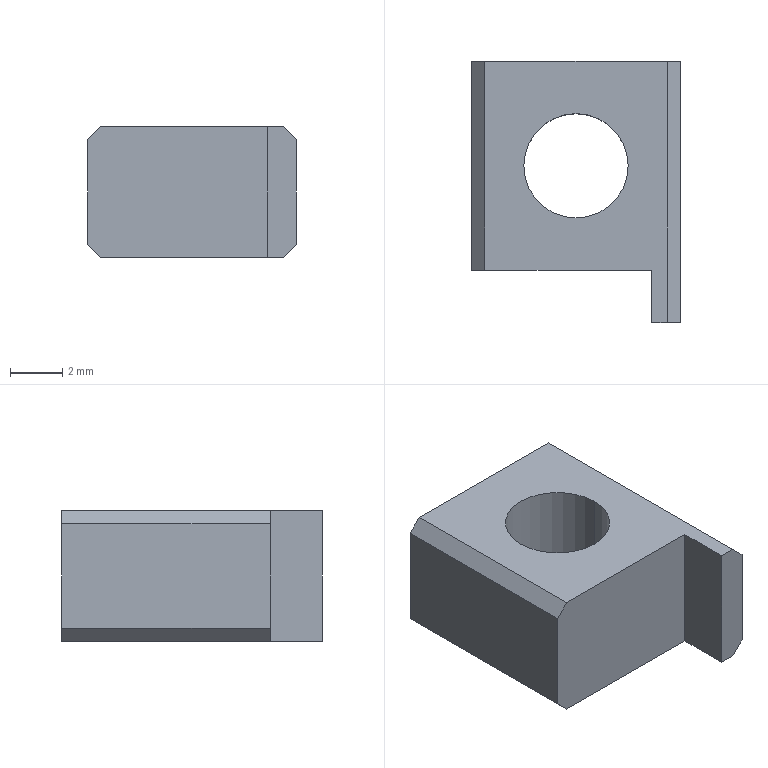Part | NX | 1 solid | 14 faces | box 8 x 10 x 5 mm | volume 263.668 mm3 | plane 12 | cylinder 2 | commonest cylinder face diameters 4 x2
STEP:
#1=CARTESIAN_POINT('',(0.5,10.,0.));
#2=VERTEX_POINT('',#1);
#3=CARTESIAN_POINT('',(7.5,10.,0.));
#4=VERTEX_POINT('',#3);
#5=CARTESIAN_POINT('',(0.,10.,0.));
#6=DIRECTION('',(1.,0.,0.));
#7=VECTOR('',#6,1000.);
#8=LINE('',#5,#7);
#9=EDGE_CURVE('',#2,#4,#8,.T.);
#10=ORIENTED_EDGE('',*,*,#9,.T.);
#11=CARTESIAN_POINT('',(7.5,0.,0.));
#12=VERTEX_POINT('',#11);
#13=CARTESIAN_POINT('',(7.5,0.,0.));
#14=DIRECTION('',(0.,-1.,0.));
#15=VECTOR('',#14,1000.);
#16=LINE('',#13,#15);
#17=EDGE_CURVE('',#4,#12,#16,.T.);
#18=ORIENTED_EDGE('',*,*,#17,.T.);
#19=CARTESIAN_POINT('',(6.9,0.,0.));
#20=VERTEX_POINT('',#19);
#21=CARTESIAN_POINT('',(0.,0.,0.));
#22=DIRECTION('',(1.,0.,0.));
#23=VECTOR('',#22,1000.);
#24=LINE('',#21,#23);
#25=EDGE_CURVE('',#20,#12,#24,.T.);
#26=ORIENTED_EDGE('',*,*,#25,.F.);
#27=CARTESIAN_POINT('',(6.9,2.,0.));
#28=VERTEX_POINT('',#27);
#29=CARTESIAN_POINT('',(6.9,0.,0.));
#30=DIRECTION('',(0.,1.,0.));
#31=VECTOR('',#30,1000.);
#32=LINE('',#29,#31);
#33=EDGE_CURVE('',#20,#28,#32,.T.);
#34=ORIENTED_EDGE('',*,*,#33,.T.);
#35=CARTESIAN_POINT('',(0.5,2.,0.));
#36=VERTEX_POINT('',#35);
#37=CARTESIAN_POINT('',(0.,2.,0.));
#38=DIRECTION('',(-1.,0.,0.));
#39=VECTOR('',#38,1000.);
#40=LINE('',#37,#39);
#41=EDGE_CURVE('',#28,#36,#40,.T.);
#42=ORIENTED_EDGE('',*,*,#41,.T.);
#43=CARTESIAN_POINT('',(0.5,0.,0.));
#44=DIRECTION('',(0.,1.,0.));
#45=VECTOR('',#44,1000.);
#46=LINE('',#43,#45);
#47=EDGE_CURVE('',#36,#2,#46,.T.);
#48=ORIENTED_EDGE('',*,*,#47,.T.);
#49=EDGE_LOOP('',(#10,#18,#26,#34,#42,#48));
#50=FACE_BOUND('',#49,.T.);
#51=CARTESIAN_POINT('',(6.,6.,0.));
#52=VERTEX_POINT('',#51);
#53=CARTESIAN_POINT('',(2.,6.,0.));
#54=VERTEX_POINT('',#53);
#55=CARTESIAN_POINT('',(4.,6.,0.));
#56=DIRECTION('',(0.,0.,-1.));
#57=DIRECTION('',(-1.,0.,0.));
#58=AXIS2_PLACEMENT_3D('',#55,#56,#57);
#59=CIRCLE('',#58,2.);
#60=EDGE_CURVE('',#52,#54,#59,.T.);
#61=ORIENTED_EDGE('',*,*,#60,.F.);
#62=CARTESIAN_POINT('',(4.,6.,0.));
#63=DIRECTION('',(0.,0.,-1.));
#64=DIRECTION('',(-1.,0.,0.));
#65=AXIS2_PLACEMENT_3D('',#62,#63,#64);
#66=CIRCLE('',#65,2.);
#67=EDGE_CURVE('',#54,#52,#66,.T.);
#68=ORIENTED_EDGE('',*,*,#67,.F.);
#69=EDGE_LOOP('',(#61,#68));
#70=FACE_BOUND('',#69,.T.);
#71=CARTESIAN_POINT('',(0.,0.,0.));
#72=DIRECTION('',(0.,0.,1.));
#73=DIRECTION('',(1.,0.,0.));
#74=AXIS2_PLACEMENT_3D('',#71,#72,#73);
#75=PLANE('',#74);
#76=ADVANCED_FACE('',(#50,#70),#75,.F.);
#77=ORIENTED_EDGE('',*,*,#33,.F.);
#78=CARTESIAN_POINT('',(6.9,0.,5.));
#79=VERTEX_POINT('',#78);
#80=CARTESIAN_POINT('',(6.9,0.,0.));
#81=DIRECTION('',(0.,0.,1.));
#82=VECTOR('',#81,1000.);
#83=LINE('',#80,#82);
#84=EDGE_CURVE('',#20,#79,#83,.T.);
#85=ORIENTED_EDGE('',*,*,#84,.T.);
#86=CARTESIAN_POINT('',(6.9,2.,5.));
#87=VERTEX_POINT('',#86);
#88=CARTESIAN_POINT('',(6.9,0.,5.));
#89=DIRECTION('',(0.,1.,0.));
#90=VECTOR('',#89,1000.);
#91=LINE('',#88,#90);
#92=EDGE_CURVE('',#79,#87,#91,.T.);
#93=ORIENTED_EDGE('',*,*,#92,.T.);
#94=CARTESIAN_POINT('',(6.9,2.,0.));
#95=DIRECTION('',(0.,0.,1.));
#96=VECTOR('',#95,1000.);
#97=LINE('',#94,#96);
#98=EDGE_CURVE('',#28,#87,#97,.T.);
#99=ORIENTED_EDGE('',*,*,#98,.F.);
#100=EDGE_LOOP('',(#77,#85,#93,#99));
#101=FACE_BOUND('',#100,.T.);
#102=CARTESIAN_POINT('',(6.9,0.,5.));
#103=DIRECTION('',(1.,0.,0.));
#104=DIRECTION('',(0.,1.,0.));
#105=AXIS2_PLACEMENT_3D('',#102,#103,#104);
#106=PLANE('',#105);
#107=ADVANCED_FACE('',(#101),#106,.F.);
#108=ORIENTED_EDGE('',*,*,#41,.F.);
#109=ORIENTED_EDGE('',*,*,#98,.T.);
#110=CARTESIAN_POINT('',(0.5,2.,5.));
#111=VERTEX_POINT('',#110);
#112=CARTESIAN_POINT('',(0.,2.,5.));
#113=DIRECTION('',(-1.,0.,0.));
#114=VECTOR('',#113,1000.);
#115=LINE('',#112,#114);
#116=EDGE_CURVE('',#87,#111,#115,.T.);
#117=ORIENTED_EDGE('',*,*,#116,.T.);
#118=CARTESIAN_POINT('',(0.,2.,4.5));
#119=VERTEX_POINT('',#118);
#120=CARTESIAN_POINT('',(-4.5,2.,0.));
#121=DIRECTION('',(-0.7071,0.,-0.7071));
#122=VECTOR('',#121,1000.);
#123=LINE('',#120,#122);
#124=EDGE_CURVE('',#111,#119,#123,.T.);
#125=ORIENTED_EDGE('',*,*,#124,.T.);
#126=CARTESIAN_POINT('',(0.,2.,0.5));
#127=VERTEX_POINT('',#126);
#128=CARTESIAN_POINT('',(0.,2.,0.));
#129=DIRECTION('',(0.,0.,-1.));
#130=VECTOR('',#129,1000.);
#131=LINE('',#128,#130);
#132=EDGE_CURVE('',#119,#127,#131,.T.);
#133=ORIENTED_EDGE('',*,*,#132,.T.);
#134=CARTESIAN_POINT('',(0.5,2.,0.));
#135=DIRECTION('',(0.7071,0.,-0.7071));
#136=VECTOR('',#135,1000.);
#137=LINE('',#134,#136);
#138=EDGE_CURVE('',#127,#36,#137,.T.);
#139=ORIENTED_EDGE('',*,*,#138,.T.);
#140=EDGE_LOOP('',(#108,#109,#117,#125,#133,#139));
#141=FACE_BOUND('',#140,.T.);
#142=CARTESIAN_POINT('',(7.,2.,5.));
#143=DIRECTION('',(0.,1.,0.));
#144=DIRECTION('',(1.,0.,0.));
#145=AXIS2_PLACEMENT_3D('',#142,#143,#144);
#146=PLANE('',#145);
#147=ADVANCED_FACE('',(#141),#146,.F.);
#148=CARTESIAN_POINT('',(0.,10.,4.5));
#149=VERTEX_POINT('',#148);
#150=CARTESIAN_POINT('',(0.,0.,4.5));
#151=DIRECTION('',(0.,-1.,0.));
#152=VECTOR('',#151,1000.);
#153=LINE('',#150,#152);
#154=EDGE_CURVE('',#149,#119,#153,.T.);
#155=ORIENTED_EDGE('',*,*,#154,.F.);
#156=CARTESIAN_POINT('',(0.,10.,0.5));
#157=VERTEX_POINT('',#156);
#158=CARTESIAN_POINT('',(0.,10.,0.));
#159=DIRECTION('',(0.,0.,-1.));
#160=VECTOR('',#159,1000.);
#161=LINE('',#158,#160);
#162=EDGE_CURVE('',#149,#157,#161,.T.);
#163=ORIENTED_EDGE('',*,*,#162,.T.);
#164=CARTESIAN_POINT('',(0.,0.,0.5));
#165=DIRECTION('',(0.,-1.,0.));
#166=VECTOR('',#165,1000.);
#167=LINE('',#164,#166);
#168=EDGE_CURVE('',#157,#127,#167,.T.);
#169=ORIENTED_EDGE('',*,*,#168,.T.);
#170=ORIENTED_EDGE('',*,*,#132,.F.);
#171=EDGE_LOOP('',(#155,#163,#169,#170));
#172=FACE_BOUND('',#171,.T.);
#173=CARTESIAN_POINT('',(0.,10.,0.));
#174=DIRECTION('',(-1.,0.,0.));
#175=DIRECTION('',(0.,0.,1.));
#176=AXIS2_PLACEMENT_3D('',#173,#174,#175);
#177=PLANE('',#176);
#178=ADVANCED_FACE('',(#172),#177,.T.);
#179=CARTESIAN_POINT('',(8.,10.,0.5));
#180=VERTEX_POINT('',#179);
#181=CARTESIAN_POINT('',(7.5,10.,0.));
#182=DIRECTION('',(-0.7071,0.,-0.7071));
#183=VECTOR('',#182,1000.);
#184=LINE('',#181,#183);
#185=EDGE_CURVE('',#180,#4,#184,.T.);
#186=ORIENTED_EDGE('',*,*,#185,.T.);
#187=ORIENTED_EDGE('',*,*,#9,.F.);
#188=CARTESIAN_POINT('',(0.5,10.,0.));
#189=DIRECTION('',(-0.7071,0.,0.7071));
#190=VECTOR('',#189,1000.);
#191=LINE('',#188,#190);
#192=EDGE_CURVE('',#2,#157,#191,.T.);
#193=ORIENTED_EDGE('',*,*,#192,.T.);
#194=ORIENTED_EDGE('',*,*,#162,.F.);
#195=CARTESIAN_POINT('',(0.5,10.,5.));
#196=VERTEX_POINT('',#195);
#197=CARTESIAN_POINT('',(-4.5,10.,0.));
#198=DIRECTION('',(-0.7071,0.,-0.7071));
#199=VECTOR('',#198,1000.);
#200=LINE('',#197,#199);
#201=EDGE_CURVE('',#196,#149,#200,.T.);
#202=ORIENTED_EDGE('',*,*,#201,.F.);
#203=CARTESIAN_POINT('',(7.5,10.,5.));
#204=VERTEX_POINT('',#203);
#205=CARTESIAN_POINT('',(0.,10.,5.));
#206=DIRECTION('',(1.,0.,0.));
#207=VECTOR('',#206,1000.);
#208=LINE('',#205,#207);
#209=EDGE_CURVE('',#196,#204,#208,.T.);
#210=ORIENTED_EDGE('',*,*,#209,.T.);
#211=CARTESIAN_POINT('',(8.,10.,4.5));
#212=VERTEX_POINT('',#211);
#213=CARTESIAN_POINT('',(12.5,10.,0.));
#214=DIRECTION('',(-0.7071,0.,0.7071));
#215=VECTOR('',#214,1000.);
#216=LINE('',#213,#215);
#217=EDGE_CURVE('',#212,#204,#216,.T.);
#218=ORIENTED_EDGE('',*,*,#217,.F.);
#219=CARTESIAN_POINT('',(8.,10.,0.));
#220=DIRECTION('',(0.,0.,1.));
#221=VECTOR('',#220,1000.);
#222=LINE('',#219,#221);
#223=EDGE_CURVE('',#180,#212,#222,.T.);
#224=ORIENTED_EDGE('',*,*,#223,.F.);
#225=EDGE_LOOP('',(#186,#187,#193,#194,#202,#210,#218,#224));
#226=FACE_BOUND('',#225,.T.);
#227=CARTESIAN_POINT('',(8.,10.,0.));
#228=DIRECTION('',(0.,1.,0.));
#229=DIRECTION('',(1.,0.,0.));
#230=AXIS2_PLACEMENT_3D('',#227,#228,#229);
#231=PLANE('',#230);
#232=ADVANCED_FACE('',(#226),#231,.T.);
#233=CARTESIAN_POINT('',(8.,0.,4.5));
#234=VERTEX_POINT('',#233);
#235=CARTESIAN_POINT('',(8.,0.,4.5));
#236=DIRECTION('',(0.,1.,0.));
#237=VECTOR('',#236,1000.);
#238=LINE('',#235,#237);
#239=EDGE_CURVE('',#234,#212,#238,.T.);
#240=ORIENTED_EDGE('',*,*,#239,.F.);
#241=CARTESIAN_POINT('',(8.,0.,0.5));
#242=VERTEX_POINT('',#241);
#243=CARTESIAN_POINT('',(8.,0.,0.));
#244=DIRECTION('',(0.,0.,-1.));
#245=VECTOR('',#244,1000.);
#246=LINE('',#243,#245);
#247=EDGE_CURVE('',#234,#242,#246,.T.);
#248=ORIENTED_EDGE('',*,*,#247,.T.);
#249=CARTESIAN_POINT('',(8.,0.,0.5));
#250=DIRECTION('',(0.,1.,0.));
#251=VECTOR('',#250,1000.);
#252=LINE('',#249,#251);
#253=EDGE_CURVE('',#242,#180,#252,.T.);
#254=ORIENTED_EDGE('',*,*,#253,.T.);
#255=ORIENTED_EDGE('',*,*,#223,.T.);
#256=EDGE_LOOP('',(#240,#248,#254,#255));
#257=FACE_BOUND('',#256,.T.);
#258=CARTESIAN_POINT('',(8.,0.,0.));
#259=DIRECTION('',(1.,0.,0.));
#260=DIRECTION('',(0.,1.,0.));
#261=AXIS2_PLACEMENT_3D('',#258,#259,#260);
#262=PLANE('',#261);
#263=ADVANCED_FACE('',(#257),#262,.T.);
#264=ORIENTED_EDGE('',*,*,#84,.F.);
#265=ORIENTED_EDGE('',*,*,#25,.T.);
#266=CARTESIAN_POINT('',(7.5,0.,0.));
#267=DIRECTION('',(-0.7071,0.,-0.7071));
#268=VECTOR('',#267,1000.);
#269=LINE('',#266,#268);
#270=EDGE_CURVE('',#242,#12,#269,.T.);
#271=ORIENTED_EDGE('',*,*,#270,.F.);
#272=ORIENTED_EDGE('',*,*,#247,.F.);
#273=CARTESIAN_POINT('',(7.5,0.,5.));
#274=VERTEX_POINT('',#273);
#275=CARTESIAN_POINT('',(12.5,0.,0.));
#276=DIRECTION('',(0.7071,0.,-0.7071));
#277=VECTOR('',#276,1000.);
#278=LINE('',#275,#277);
#279=EDGE_CURVE('',#274,#234,#278,.T.);
#280=ORIENTED_EDGE('',*,*,#279,.F.);
#281=CARTESIAN_POINT('',(0.,0.,5.));
#282=DIRECTION('',(1.,0.,0.));
#283=VECTOR('',#282,1000.);
#284=LINE('',#281,#283);
#285=EDGE_CURVE('',#79,#274,#284,.T.);
#286=ORIENTED_EDGE('',*,*,#285,.F.);
#287=EDGE_LOOP('',(#264,#265,#271,#272,#280,#286));
#288=FACE_BOUND('',#287,.T.);
#289=CARTESIAN_POINT('',(0.,0.,0.));
#290=DIRECTION('',(0.,-1.,0.));
#291=DIRECTION('',(0.,0.,-1.));
#292=AXIS2_PLACEMENT_3D('',#289,#290,#291);
#293=PLANE('',#292);
#294=ADVANCED_FACE('',(#288),#293,.T.);
#295=ORIENTED_EDGE('',*,*,#209,.F.);
#296=CARTESIAN_POINT('',(0.5,0.,5.));
#297=DIRECTION('',(0.,1.,0.));
#298=VECTOR('',#297,1000.);
#299=LINE('',#296,#298);
#300=EDGE_CURVE('',#111,#196,#299,.T.);
#301=ORIENTED_EDGE('',*,*,#300,.F.);
#302=ORIENTED_EDGE('',*,*,#116,.F.);
#303=ORIENTED_EDGE('',*,*,#92,.F.);
#304=ORIENTED_EDGE('',*,*,#285,.T.);
#305=CARTESIAN_POINT('',(7.5,0.,5.));
#306=DIRECTION('',(0.,-1.,0.));
#307=VECTOR('',#306,1000.);
#308=LINE('',#305,#307);
#309=EDGE_CURVE('',#204,#274,#308,.T.);
#310=ORIENTED_EDGE('',*,*,#309,.F.);
#311=EDGE_LOOP('',(#295,#301,#302,#303,#304,#310));
#312=FACE_BOUND('',#311,.T.);
#313=CARTESIAN_POINT('',(2.,6.,5.));
#314=VERTEX_POINT('',#313);
#315=CARTESIAN_POINT('',(6.,6.,5.));
#316=VERTEX_POINT('',#315);
#317=CARTESIAN_POINT('',(4.,6.,5.));
#318=DIRECTION('',(0.,0.,-1.));
#319=DIRECTION('',(-1.,0.,0.));
#320=AXIS2_PLACEMENT_3D('',#317,#318,#319);
#321=CIRCLE('',#320,2.);
#322=EDGE_CURVE('',#314,#316,#321,.T.);
#323=ORIENTED_EDGE('',*,*,#322,.T.);
#324=CARTESIAN_POINT('',(4.,6.,5.));
#325=DIRECTION('',(0.,0.,-1.));
#326=DIRECTION('',(-1.,0.,0.));
#327=AXIS2_PLACEMENT_3D('',#324,#325,#326);
#328=CIRCLE('',#327,2.);
#329=EDGE_CURVE('',#316,#314,#328,.T.);
#330=ORIENTED_EDGE('',*,*,#329,.T.);
#331=EDGE_LOOP('',(#323,#330));
#332=FACE_BOUND('',#331,.T.);
#333=CARTESIAN_POINT('',(0.,0.,5.));
#334=DIRECTION('',(0.,0.,1.));
#335=DIRECTION('',(1.,0.,0.));
#336=AXIS2_PLACEMENT_3D('',#333,#334,#335);
#337=PLANE('',#336);
#338=ADVANCED_FACE('',(#312,#332),#337,.T.);
#339=ORIENTED_EDGE('',*,*,#322,.F.);
#340=CARTESIAN_POINT('',(2.,6.,5.));
#341=DIRECTION('',(0.,0.,-1.));
#342=VECTOR('',#341,1000.);
#343=LINE('',#340,#342);
#344=EDGE_CURVE('',#54,#314,#343,.F.);
#345=ORIENTED_EDGE('',*,*,#344,.F.);
#346=ORIENTED_EDGE('',*,*,#67,.T.);
#347=CARTESIAN_POINT('',(6.,6.,5.));
#348=DIRECTION('',(0.,0.,-1.));
#349=VECTOR('',#348,1000.);
#350=LINE('',#347,#349);
#351=EDGE_CURVE('',#52,#316,#350,.F.);
#352=ORIENTED_EDGE('',*,*,#351,.T.);
#353=EDGE_LOOP('',(#339,#345,#346,#352));
#354=FACE_BOUND('',#353,.T.);
#355=CARTESIAN_POINT('',(4.,6.,5.));
#356=DIRECTION('',(0.,0.,-1.));
#357=DIRECTION('',(-1.,0.,0.));
#358=AXIS2_PLACEMENT_3D('',#355,#356,#357);
#359=CYLINDRICAL_SURFACE('',#358,2.);
#360=ADVANCED_FACE('',(#354),#359,.F.);
#361=ORIENTED_EDGE('',*,*,#201,.T.);
#362=ORIENTED_EDGE('',*,*,#154,.T.);
#363=ORIENTED_EDGE('',*,*,#124,.F.);
#364=ORIENTED_EDGE('',*,*,#300,.T.);
#365=EDGE_LOOP('',(#361,#362,#363,#364));
#366=FACE_BOUND('',#365,.T.);
#367=CARTESIAN_POINT('',(0.25,6.,4.75));
#368=DIRECTION('',(-0.7071,0.,0.7071));
#369=DIRECTION('',(0.,1.,0.));
#370=AXIS2_PLACEMENT_3D('',#367,#368,#369);
#371=PLANE('',#370);
#372=ADVANCED_FACE('',(#366),#371,.T.);
#373=ORIENTED_EDGE('',*,*,#217,.T.);
#374=ORIENTED_EDGE('',*,*,#309,.T.);
#375=ORIENTED_EDGE('',*,*,#279,.T.);
#376=ORIENTED_EDGE('',*,*,#239,.T.);
#377=EDGE_LOOP('',(#373,#374,#375,#376));
#378=FACE_BOUND('',#377,.T.);
#379=CARTESIAN_POINT('',(7.75,5.,4.75));
#380=DIRECTION('',(0.7071,0.,0.7071));
#381=DIRECTION('',(0.,-1.,0.));
#382=AXIS2_PLACEMENT_3D('',#379,#380,#381);
#383=PLANE('',#382);
#384=ADVANCED_FACE('',(#378),#383,.T.);
#385=ORIENTED_EDGE('',*,*,#185,.F.);
#386=ORIENTED_EDGE('',*,*,#253,.F.);
#387=ORIENTED_EDGE('',*,*,#270,.T.);
#388=ORIENTED_EDGE('',*,*,#17,.F.);
#389=EDGE_LOOP('',(#385,#386,#387,#388));
#390=FACE_BOUND('',#389,.T.);
#391=CARTESIAN_POINT('',(7.75,5.,0.25));
#392=DIRECTION('',(0.7071,0.,-0.7071));
#393=DIRECTION('',(0.,-1.,0.));
#394=AXIS2_PLACEMENT_3D('',#391,#392,#393);
#395=PLANE('',#394);
#396=ADVANCED_FACE('',(#390),#395,.T.);
#397=ORIENTED_EDGE('',*,*,#192,.F.);
#398=ORIENTED_EDGE('',*,*,#47,.F.);
#399=ORIENTED_EDGE('',*,*,#138,.F.);
#400=ORIENTED_EDGE('',*,*,#168,.F.);
#401=EDGE_LOOP('',(#397,#398,#399,#400));
#402=FACE_BOUND('',#401,.T.);
#403=CARTESIAN_POINT('',(0.25,6.,0.25));
#404=DIRECTION('',(-0.7071,0.,-0.7071));
#405=DIRECTION('',(-0.7071,0.,0.7071));
#406=AXIS2_PLACEMENT_3D('',#403,#404,#405);
#407=PLANE('',#406);
#408=ADVANCED_FACE('',(#402),#407,.T.);
#409=ORIENTED_EDGE('',*,*,#60,.T.);
#410=ORIENTED_EDGE('',*,*,#344,.T.);
#411=ORIENTED_EDGE('',*,*,#329,.F.);
#412=ORIENTED_EDGE('',*,*,#351,.F.);
#413=EDGE_LOOP('',(#409,#410,#411,#412));
#414=FACE_BOUND('',#413,.T.);
#415=CARTESIAN_POINT('',(4.,6.,5.));
#416=DIRECTION('',(0.,0.,-1.));
#417=DIRECTION('',(-1.,0.,0.));
#418=AXIS2_PLACEMENT_3D('',#415,#416,#417);
#419=CYLINDRICAL_SURFACE('',#418,2.);
#420=ADVANCED_FACE('',(#414),#419,.F.);
#421=CLOSED_SHELL('',(#76,#107,#147,#178,#232,#263,#294,#338,#360,#372,#384,#396,#408,#420));
#422=MANIFOLD_SOLID_BREP('',#421);
#423=(LENGTH_UNIT()NAMED_UNIT(*)SI_UNIT(.MILLI.,.METRE.));
#424=UNCERTAINTY_MEASURE_WITH_UNIT(LENGTH_MEASURE(0.00001),#423,'','');
#425=(NAMED_UNIT(*)PLANE_ANGLE_UNIT()SI_UNIT($,.RADIAN.));
#426=(NAMED_UNIT(*)SI_UNIT($,.STERADIAN.)SOLID_ANGLE_UNIT());
#427=(GEOMETRIC_REPRESENTATION_CONTEXT(3)GLOBAL_UNCERTAINTY_ASSIGNED_CONTEXT((#424))GLOBAL_UNIT_ASSIGNED_CONTEXT((#423,#425,#426))REPRESENTATION_CONTEXT('',''));
#428=ADVANCED_BREP_SHAPE_REPRESENTATION('',(#422),#427);